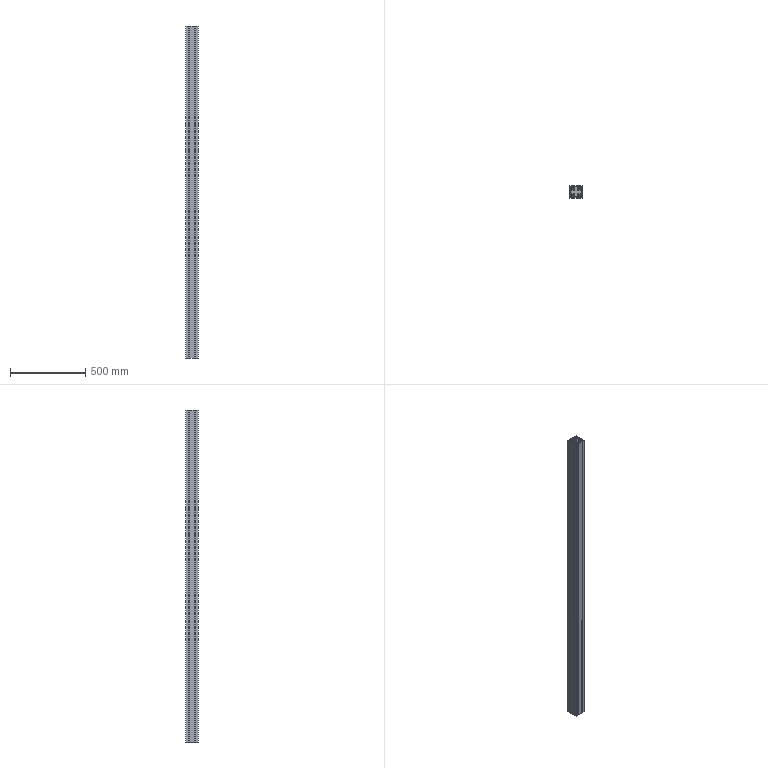Part | NX | features BREP 1 | 1 solid | 139 faces | box 80 x 80 x 2200 mm | volume 9449266 mm3 | plane 123 | cylinder 16 | commonest cylinder face diameters 6.8 x16